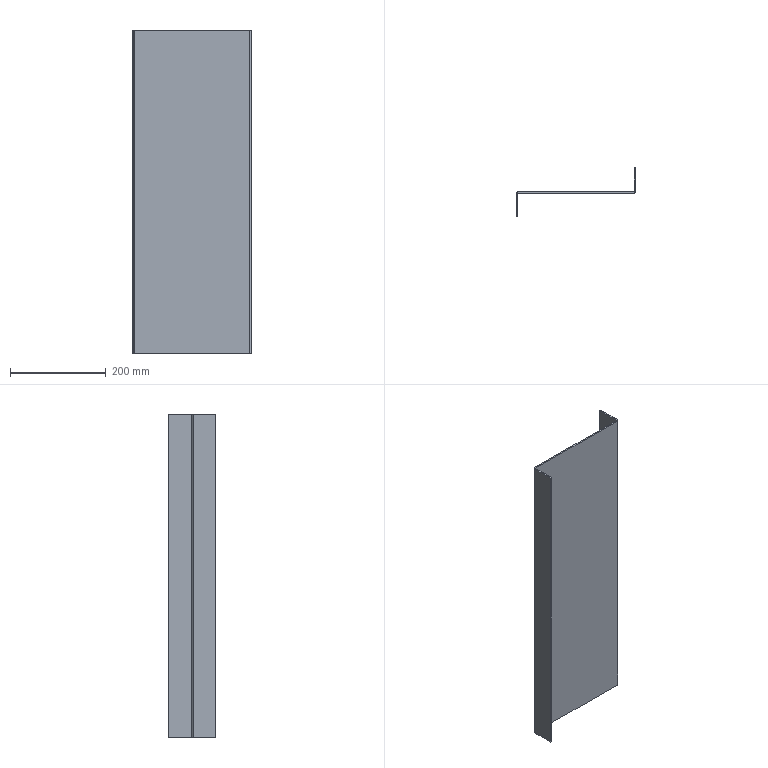Part | STEP file | 粉仓楼梯踏Plate 1 | 1 solid | 14 faces | box 248 x 100 x 674 mm | volume 693251 mm3 | plane 10 | cylinder 4 | commonest cylinder face diameters 2 x2 8 x2
STEP:
#1=CARTESIAN_POINT('',(0.,0.,0.));
#2=DIRECTION('',(0.,0.,1.));
#3=DIRECTION('',(1.,0.,0.));
#4=AXIS2_PLACEMENT_3D('',#1,#2,#3);
#5=CARTESIAN_POINT('',(3.,1.,-337.));
#6=VERTEX_POINT('',#5);
#7=CARTESIAN_POINT('',(3.,50.,-337.));
#8=VERTEX_POINT('',#7);
#9=CARTESIAN_POINT('',(3.,1.,-337.));
#10=DIRECTION('',(0.,1.,0.));
#11=VECTOR('',#10,1.);
#12=LINE('',#9,#11);
#13=CARTESIAN_POINT('',(3.,1.,337.));
#14=DIRECTION('',(-1.,0.,0.));
#15=DIRECTION('',(0.,0.,1.));
#16=AXIS2_PLACEMENT_3D('',#13,#14,#15);
#17=PLANE('',#16);
#18=CARTESIAN_POINT('',(-674.,0.));
#19=DIRECTION('',(0.,1.));
#20=VECTOR('',#19,1.);
#21=LINE('',#18,#20);
#22=(GEOMETRIC_REPRESENTATION_CONTEXT(2)PARAMETRIC_REPRESENTATION_CONTEXT()REPRESENTATION_CONTEXT('',''));
#23=DEFINITIONAL_REPRESENTATION('',(#21),#22);
#24=PCURVE('',#17,#23);
#25=CARTESIAN_POINT('',(-1.,1.,-337.));
#26=DIRECTION('',(0.,0.,1.));
#27=DIRECTION('',(1.,0.,0.));
#28=AXIS2_PLACEMENT_3D('',#25,#26,#27);
#29=PLANE('',#28);
#30=CARTESIAN_POINT('',(4.,0.));
#31=DIRECTION('',(0.,1.));
#32=VECTOR('',#31,1.);
#33=LINE('',#30,#32);
#34=(GEOMETRIC_REPRESENTATION_CONTEXT(2)PARAMETRIC_REPRESENTATION_CONTEXT()REPRESENTATION_CONTEXT('',''));
#35=DEFINITIONAL_REPRESENTATION('',(#33),#34);
#36=PCURVE('',#29,#35);
#37=SURFACE_CURVE('',#12,(#24,#36),.PCURVE_S1.);
#38=EDGE_CURVE('',#6,#8,#37,.T.);
#39=ORIENTED_EDGE('',*,*,#38,.T.);
#40=CARTESIAN_POINT('',(3.,50.,337.));
#41=VERTEX_POINT('',#40);
#42=CARTESIAN_POINT('',(3.,50.,337.));
#43=DIRECTION('',(0.,0.,-1.));
#44=VECTOR('',#43,1.);
#45=LINE('',#42,#44);
#46=CARTESIAN_POINT('',(0.,49.));
#47=DIRECTION('',(-1.,0.));
#48=VECTOR('',#47,1.);
#49=LINE('',#46,#48);
#50=(GEOMETRIC_REPRESENTATION_CONTEXT(2)PARAMETRIC_REPRESENTATION_CONTEXT()REPRESENTATION_CONTEXT('',''));
#51=DEFINITIONAL_REPRESENTATION('',(#49),#50);
#52=PCURVE('',#17,#51);
#53=CARTESIAN_POINT('',(0.,50.,337.));
#54=DIRECTION('',(0.,1.,0.));
#55=DIRECTION('',(0.,0.,1.));
#56=AXIS2_PLACEMENT_3D('',#53,#54,#55);
#57=PLANE('',#56);
#58=CARTESIAN_POINT('',(0.,3.));
#59=DIRECTION('',(-1.,0.));
#60=VECTOR('',#59,1.);
#61=LINE('',#58,#60);
#62=(GEOMETRIC_REPRESENTATION_CONTEXT(2)PARAMETRIC_REPRESENTATION_CONTEXT()REPRESENTATION_CONTEXT('',''));
#63=DEFINITIONAL_REPRESENTATION('',(#61),#62);
#64=PCURVE('',#57,#63);
#65=SURFACE_CURVE('',#45,(#52,#64),.PCURVE_S1.);
#66=EDGE_CURVE('',#41,#8,#65,.T.);
#67=ORIENTED_EDGE('',*,*,#66,.F.);
#68=CARTESIAN_POINT('',(3.,1.,337.));
#69=VERTEX_POINT('',#68);
#70=CARTESIAN_POINT('',(3.,1.,337.));
#71=DIRECTION('',(0.,1.,0.));
#72=VECTOR('',#71,1.);
#73=LINE('',#70,#72);
#74=CARTESIAN_POINT('',(0.,0.));
#75=DIRECTION('',(0.,1.));
#76=VECTOR('',#75,1.);
#77=LINE('',#74,#76);
#78=(GEOMETRIC_REPRESENTATION_CONTEXT(2)PARAMETRIC_REPRESENTATION_CONTEXT()REPRESENTATION_CONTEXT('',''));
#79=DEFINITIONAL_REPRESENTATION('',(#77),#78);
#80=PCURVE('',#17,#79);
#81=CARTESIAN_POINT('',(-1.,1.,337.));
#82=DIRECTION('',(0.,0.,1.));
#83=DIRECTION('',(1.,0.,0.));
#84=AXIS2_PLACEMENT_3D('',#81,#82,#83);
#85=PLANE('',#84);
#86=CARTESIAN_POINT('',(4.,0.));
#87=DIRECTION('',(0.,1.));
#88=VECTOR('',#87,1.);
#89=LINE('',#86,#88);
#90=(GEOMETRIC_REPRESENTATION_CONTEXT(2)PARAMETRIC_REPRESENTATION_CONTEXT()REPRESENTATION_CONTEXT('',''));
#91=DEFINITIONAL_REPRESENTATION('',(#89),#90);
#92=PCURVE('',#85,#91);
#93=SURFACE_CURVE('',#73,(#80,#92),.PCURVE_S1.);
#94=EDGE_CURVE('',#69,#41,#93,.T.);
#95=ORIENTED_EDGE('',*,*,#94,.F.);
#96=CARTESIAN_POINT('',(3.,1.,337.));
#97=DIRECTION('',(0.,0.,-1.));
#98=VECTOR('',#97,1.);
#99=LINE('',#96,#98);
#100=CARTESIAN_POINT('',(0.,0.));
#101=DIRECTION('',(-1.,0.));
#102=VECTOR('',#101,1.);
#103=LINE('',#100,#102);
#104=(GEOMETRIC_REPRESENTATION_CONTEXT(2)PARAMETRIC_REPRESENTATION_CONTEXT()REPRESENTATION_CONTEXT('',''));
#105=DEFINITIONAL_REPRESENTATION('',(#103),#104);
#106=PCURVE('',#17,#105);
#107=CARTESIAN_POINT('',(-1.,1.,337.));
#108=DIRECTION('',(0.,0.,-1.));
#109=DIRECTION('',(-1.,0.,0.));
#110=AXIS2_PLACEMENT_3D('',#107,#108,#109);
#111=CYLINDRICAL_SURFACE('',#110,4.);
#112=CARTESIAN_POINT('',(3.142,0.));
#113=DIRECTION('',(0.,1.));
#114=VECTOR('',#113,1.);
#115=LINE('',#112,#114);
#116=(GEOMETRIC_REPRESENTATION_CONTEXT(2)PARAMETRIC_REPRESENTATION_CONTEXT()REPRESENTATION_CONTEXT('',''));
#117=DEFINITIONAL_REPRESENTATION('',(#115),#116);
#118=PCURVE('',#111,#117);
#119=SURFACE_CURVE('',#99,(#106,#118),.PCURVE_S1.);
#120=EDGE_CURVE('',#69,#6,#119,.T.);
#121=ORIENTED_EDGE('',*,*,#120,.T.);
#122=EDGE_LOOP('',(#39,#67,#95,#121));
#123=FACE_BOUND('',#122,.T.);
#124=ADVANCED_FACE('',(#123),#17,.F.);
#125=CARTESIAN_POINT('',(0.,50.,-337.));
#126=VERTEX_POINT('',#125);
#127=CARTESIAN_POINT('',(0.,50.,-337.));
#128=DIRECTION('',(1.,0.,0.));
#129=VECTOR('',#128,1.);
#130=LINE('',#127,#129);
#131=CARTESIAN_POINT('',(-674.,0.));
#132=DIRECTION('',(0.,1.));
#133=VECTOR('',#132,1.);
#134=LINE('',#131,#133);
#135=(GEOMETRIC_REPRESENTATION_CONTEXT(2)PARAMETRIC_REPRESENTATION_CONTEXT()REPRESENTATION_CONTEXT('',''));
#136=DEFINITIONAL_REPRESENTATION('',(#134),#135);
#137=PCURVE('',#57,#136);
#138=CARTESIAN_POINT('',(1.,49.));
#139=DIRECTION('',(1.,0.));
#140=VECTOR('',#139,1.);
#141=LINE('',#138,#140);
#142=(GEOMETRIC_REPRESENTATION_CONTEXT(2)PARAMETRIC_REPRESENTATION_CONTEXT()REPRESENTATION_CONTEXT('',''));
#143=DEFINITIONAL_REPRESENTATION('',(#141),#142);
#144=PCURVE('',#29,#143);
#145=SURFACE_CURVE('',#130,(#137,#144),.PCURVE_S1.);
#146=EDGE_CURVE('',#126,#8,#145,.T.);
#147=ORIENTED_EDGE('',*,*,#146,.F.);
#148=CARTESIAN_POINT('',(0.,50.,337.));
#149=VERTEX_POINT('',#148);
#150=CARTESIAN_POINT('',(0.,50.,337.));
#151=DIRECTION('',(0.,0.,-1.));
#152=VECTOR('',#151,1.);
#153=LINE('',#150,#152);
#154=CARTESIAN_POINT('',(0.,0.));
#155=DIRECTION('',(-1.,0.));
#156=VECTOR('',#155,1.);
#157=LINE('',#154,#156);
#158=(GEOMETRIC_REPRESENTATION_CONTEXT(2)PARAMETRIC_REPRESENTATION_CONTEXT()REPRESENTATION_CONTEXT('',''));
#159=DEFINITIONAL_REPRESENTATION('',(#157),#158);
#160=PCURVE('',#57,#159);
#161=CARTESIAN_POINT('',(0.,1.,337.));
#162=DIRECTION('',(-1.,0.,0.));
#163=DIRECTION('',(0.,0.,1.));
#164=AXIS2_PLACEMENT_3D('',#161,#162,#163);
#165=PLANE('',#164);
#166=CARTESIAN_POINT('',(0.,49.));
#167=DIRECTION('',(-1.,0.));
#168=VECTOR('',#167,1.);
#169=LINE('',#166,#168);
#170=(GEOMETRIC_REPRESENTATION_CONTEXT(2)PARAMETRIC_REPRESENTATION_CONTEXT()REPRESENTATION_CONTEXT('',''));
#171=DEFINITIONAL_REPRESENTATION('',(#169),#170);
#172=PCURVE('',#165,#171);
#173=SURFACE_CURVE('',#153,(#160,#172),.PCURVE_S1.);
#174=EDGE_CURVE('',#149,#126,#173,.T.);
#175=ORIENTED_EDGE('',*,*,#174,.F.);
#176=CARTESIAN_POINT('',(0.,50.,337.));
#177=DIRECTION('',(1.,0.,0.));
#178=VECTOR('',#177,1.);
#179=LINE('',#176,#178);
#180=CARTESIAN_POINT('',(0.,0.));
#181=DIRECTION('',(0.,1.));
#182=VECTOR('',#181,1.);
#183=LINE('',#180,#182);
#184=(GEOMETRIC_REPRESENTATION_CONTEXT(2)PARAMETRIC_REPRESENTATION_CONTEXT()REPRESENTATION_CONTEXT('',''));
#185=DEFINITIONAL_REPRESENTATION('',(#183),#184);
#186=PCURVE('',#57,#185);
#187=CARTESIAN_POINT('',(1.,49.));
#188=DIRECTION('',(1.,0.));
#189=VECTOR('',#188,1.);
#190=LINE('',#187,#189);
#191=(GEOMETRIC_REPRESENTATION_CONTEXT(2)PARAMETRIC_REPRESENTATION_CONTEXT()REPRESENTATION_CONTEXT('',''));
#192=DEFINITIONAL_REPRESENTATION('',(#190),#191);
#193=PCURVE('',#85,#192);
#194=SURFACE_CURVE('',#179,(#186,#193),.PCURVE_S1.);
#195=EDGE_CURVE('',#149,#41,#194,.T.);
#196=ORIENTED_EDGE('',*,*,#195,.T.);
#197=ORIENTED_EDGE('',*,*,#66,.T.);
#198=EDGE_LOOP('',(#147,#175,#196,#197));
#199=FACE_BOUND('',#198,.T.);
#200=ADVANCED_FACE('',(#199),#57,.T.);
#201=CARTESIAN_POINT('',(0.,1.,-337.));
#202=VERTEX_POINT('',#201);
#203=CARTESIAN_POINT('',(0.,1.,-337.));
#204=DIRECTION('',(0.,1.,0.));
#205=VECTOR('',#204,1.);
#206=LINE('',#203,#205);
#207=CARTESIAN_POINT('',(-674.,0.));
#208=DIRECTION('',(0.,1.));
#209=VECTOR('',#208,1.);
#210=LINE('',#207,#209);
#211=(GEOMETRIC_REPRESENTATION_CONTEXT(2)PARAMETRIC_REPRESENTATION_CONTEXT()REPRESENTATION_CONTEXT('',''));
#212=DEFINITIONAL_REPRESENTATION('',(#210),#211);
#213=PCURVE('',#165,#212);
#214=CARTESIAN_POINT('',(1.,0.));
#215=DIRECTION('',(0.,1.));
#216=VECTOR('',#215,1.);
#217=LINE('',#214,#216);
#218=(GEOMETRIC_REPRESENTATION_CONTEXT(2)PARAMETRIC_REPRESENTATION_CONTEXT()REPRESENTATION_CONTEXT('',''));
#219=DEFINITIONAL_REPRESENTATION('',(#217),#218);
#220=PCURVE('',#29,#219);
#221=SURFACE_CURVE('',#206,(#213,#220),.PCURVE_S1.);
#222=EDGE_CURVE('',#202,#126,#221,.T.);
#223=ORIENTED_EDGE('',*,*,#222,.F.);
#224=CARTESIAN_POINT('',(0.,1.,337.));
#225=VERTEX_POINT('',#224);
#226=CARTESIAN_POINT('',(0.,1.,337.));
#227=DIRECTION('',(0.,0.,-1.));
#228=VECTOR('',#227,1.);
#229=LINE('',#226,#228);
#230=CARTESIAN_POINT('',(0.,0.));
#231=DIRECTION('',(-1.,0.));
#232=VECTOR('',#231,1.);
#233=LINE('',#230,#232);
#234=(GEOMETRIC_REPRESENTATION_CONTEXT(2)PARAMETRIC_REPRESENTATION_CONTEXT()REPRESENTATION_CONTEXT('',''));
#235=DEFINITIONAL_REPRESENTATION('',(#233),#234);
#236=PCURVE('',#165,#235);
#237=CARTESIAN_POINT('',(-1.,1.,337.));
#238=DIRECTION('',(0.,0.,-1.));
#239=DIRECTION('',(-1.,0.,0.));
#240=AXIS2_PLACEMENT_3D('',#237,#238,#239);
#241=CYLINDRICAL_SURFACE('',#240,1.);
#242=CARTESIAN_POINT('',(3.142,0.));
#243=DIRECTION('',(0.,1.));
#244=VECTOR('',#243,1.);
#245=LINE('',#242,#244);
#246=(GEOMETRIC_REPRESENTATION_CONTEXT(2)PARAMETRIC_REPRESENTATION_CONTEXT()REPRESENTATION_CONTEXT('',''));
#247=DEFINITIONAL_REPRESENTATION('',(#245),#246);
#248=PCURVE('',#241,#247);
#249=SURFACE_CURVE('',#229,(#236,#248),.PCURVE_S1.);
#250=EDGE_CURVE('',#225,#202,#249,.T.);
#251=ORIENTED_EDGE('',*,*,#250,.F.);
#252=CARTESIAN_POINT('',(0.,1.,337.));
#253=DIRECTION('',(0.,1.,0.));
#254=VECTOR('',#253,1.);
#255=LINE('',#252,#254);
#256=CARTESIAN_POINT('',(0.,0.));
#257=DIRECTION('',(0.,1.));
#258=VECTOR('',#257,1.);
#259=LINE('',#256,#258);
#260=(GEOMETRIC_REPRESENTATION_CONTEXT(2)PARAMETRIC_REPRESENTATION_CONTEXT()REPRESENTATION_CONTEXT('',''));
#261=DEFINITIONAL_REPRESENTATION('',(#259),#260);
#262=PCURVE('',#165,#261);
#263=CARTESIAN_POINT('',(1.,0.));
#264=DIRECTION('',(0.,1.));
#265=VECTOR('',#264,1.);
#266=LINE('',#263,#265);
#267=(GEOMETRIC_REPRESENTATION_CONTEXT(2)PARAMETRIC_REPRESENTATION_CONTEXT()REPRESENTATION_CONTEXT('',''));
#268=DEFINITIONAL_REPRESENTATION('',(#266),#267);
#269=PCURVE('',#85,#268);
#270=SURFACE_CURVE('',#255,(#262,#269),.PCURVE_S1.);
#271=EDGE_CURVE('',#225,#149,#270,.T.);
#272=ORIENTED_EDGE('',*,*,#271,.T.);
#273=ORIENTED_EDGE('',*,*,#174,.T.);
#274=EDGE_LOOP('',(#223,#251,#272,#273));
#275=FACE_BOUND('',#274,.T.);
#276=ADVANCED_FACE('',(#275),#165,.T.);
#277=ORIENTED_EDGE('',*,*,#250,.F.);
#278=CARTESIAN_POINT('',(-1.,0.,337.));
#279=VERTEX_POINT('',#278);
#280=CARTESIAN_POINT('',(-1.,1.,337.));
#281=DIRECTION('',(0.,0.,1.));
#282=DIRECTION('',(1.,0.,0.));
#283=AXIS2_PLACEMENT_3D('',#280,#281,#282);
#284=CIRCLE('',#283,1.);
#285=CARTESIAN_POINT('',(9.425,0.));
#286=DIRECTION('',(-1.,0.));
#287=VECTOR('',#286,1.);
#288=LINE('',#285,#287);
#289=(GEOMETRIC_REPRESENTATION_CONTEXT(2)PARAMETRIC_REPRESENTATION_CONTEXT()REPRESENTATION_CONTEXT('',''));
#290=DEFINITIONAL_REPRESENTATION('',(#288),#289);
#291=PCURVE('',#241,#290);
#292=CARTESIAN_POINT('',(0.,0.));
#293=DIRECTION('',(1.,0.));
#294=AXIS2_PLACEMENT_2D('',#292,#293);
#295=CIRCLE('',#294,1.);
#296=(GEOMETRIC_REPRESENTATION_CONTEXT(2)PARAMETRIC_REPRESENTATION_CONTEXT()REPRESENTATION_CONTEXT('',''));
#297=DEFINITIONAL_REPRESENTATION('',(#295),#296);
#298=PCURVE('',#85,#297);
#299=SURFACE_CURVE('',#284,(#291,#298),.PCURVE_S1.);
#300=EDGE_CURVE('',#279,#225,#299,.T.);
#301=ORIENTED_EDGE('',*,*,#300,.F.);
#302=CARTESIAN_POINT('',(-1.,0.,-337.));
#303=VERTEX_POINT('',#302);
#304=CARTESIAN_POINT('',(-1.,0.,337.));
#305=DIRECTION('',(0.,0.,-1.));
#306=VECTOR('',#305,1.);
#307=LINE('',#304,#306);
#308=CARTESIAN_POINT('',(4.712,0.));
#309=DIRECTION('',(0.,1.));
#310=VECTOR('',#309,1.);
#311=LINE('',#308,#310);
#312=(GEOMETRIC_REPRESENTATION_CONTEXT(2)PARAMETRIC_REPRESENTATION_CONTEXT()REPRESENTATION_CONTEXT('',''));
#313=DEFINITIONAL_REPRESENTATION('',(#311),#312);
#314=PCURVE('',#241,#313);
#315=CARTESIAN_POINT('',(-241.,0.,337.));
#316=DIRECTION('',(0.,1.,0.));
#317=DIRECTION('',(0.,0.,1.));
#318=AXIS2_PLACEMENT_3D('',#315,#316,#317);
#319=PLANE('',#318);
#320=CARTESIAN_POINT('',(0.,240.));
#321=DIRECTION('',(-1.,0.));
#322=VECTOR('',#321,1.);
#323=LINE('',#320,#322);
#324=(GEOMETRIC_REPRESENTATION_CONTEXT(2)PARAMETRIC_REPRESENTATION_CONTEXT()REPRESENTATION_CONTEXT('',''));
#325=DEFINITIONAL_REPRESENTATION('',(#323),#324);
#326=PCURVE('',#319,#325);
#327=SURFACE_CURVE('',#307,(#314,#326),.PCURVE_S1.);
#328=EDGE_CURVE('',#279,#303,#327,.T.);
#329=ORIENTED_EDGE('',*,*,#328,.T.);
#330=CARTESIAN_POINT('',(-1.,1.,-337.));
#331=DIRECTION('',(0.,0.,1.));
#332=DIRECTION('',(1.,0.,0.));
#333=AXIS2_PLACEMENT_3D('',#330,#331,#332);
#334=CIRCLE('',#333,1.);
#335=CARTESIAN_POINT('',(9.425,674.));
#336=DIRECTION('',(-1.,0.));
#337=VECTOR('',#336,1.);
#338=LINE('',#335,#337);
#339=(GEOMETRIC_REPRESENTATION_CONTEXT(2)PARAMETRIC_REPRESENTATION_CONTEXT()REPRESENTATION_CONTEXT('',''));
#340=DEFINITIONAL_REPRESENTATION('',(#338),#339);
#341=PCURVE('',#241,#340);
#342=CARTESIAN_POINT('',(0.,0.));
#343=DIRECTION('',(1.,0.));
#344=AXIS2_PLACEMENT_2D('',#342,#343);
#345=CIRCLE('',#344,1.);
#346=(GEOMETRIC_REPRESENTATION_CONTEXT(2)PARAMETRIC_REPRESENTATION_CONTEXT()REPRESENTATION_CONTEXT('',''));
#347=DEFINITIONAL_REPRESENTATION('',(#345),#346);
#348=PCURVE('',#29,#347);
#349=SURFACE_CURVE('',#334,(#341,#348),.PCURVE_S1.);
#350=EDGE_CURVE('',#303,#202,#349,.T.);
#351=ORIENTED_EDGE('',*,*,#350,.T.);
#352=EDGE_LOOP('',(#277,#301,#329,#351));
#353=FACE_BOUND('',#352,.F.);
#354=ADVANCED_FACE('',(#353),#241,.F.);
#355=CARTESIAN_POINT('',(-241.,0.,-337.));
#356=VERTEX_POINT('',#355);
#357=CARTESIAN_POINT('',(-241.,0.,-337.));
#358=DIRECTION('',(1.,0.,0.));
#359=VECTOR('',#358,1.);
#360=LINE('',#357,#359);
#361=CARTESIAN_POINT('',(-674.,0.));
#362=DIRECTION('',(0.,1.));
#363=VECTOR('',#362,1.);
#364=LINE('',#361,#363);
#365=(GEOMETRIC_REPRESENTATION_CONTEXT(2)PARAMETRIC_REPRESENTATION_CONTEXT()REPRESENTATION_CONTEXT('',''));
#366=DEFINITIONAL_REPRESENTATION('',(#364),#365);
#367=PCURVE('',#319,#366);
#368=CARTESIAN_POINT('',(-240.,-1.));
#369=DIRECTION('',(1.,0.));
#370=VECTOR('',#369,1.);
#371=LINE('',#368,#370);
#372=(GEOMETRIC_REPRESENTATION_CONTEXT(2)PARAMETRIC_REPRESENTATION_CONTEXT()REPRESENTATION_CONTEXT('',''));
#373=DEFINITIONAL_REPRESENTATION('',(#371),#372);
#374=PCURVE('',#29,#373);
#375=SURFACE_CURVE('',#360,(#367,#374),.PCURVE_S1.);
#376=EDGE_CURVE('',#356,#303,#375,.T.);
#377=ORIENTED_EDGE('',*,*,#376,.F.);
#378=CARTESIAN_POINT('',(-241.,0.,337.));
#379=VERTEX_POINT('',#378);
#380=CARTESIAN_POINT('',(-241.,0.,337.));
#381=DIRECTION('',(0.,0.,-1.));
#382=VECTOR('',#381,1.);
#383=LINE('',#380,#382);
#384=CARTESIAN_POINT('',(0.,0.));
#385=DIRECTION('',(-1.,0.));
#386=VECTOR('',#385,1.);
#387=LINE('',#384,#386);
#388=(GEOMETRIC_REPRESENTATION_CONTEXT(2)PARAMETRIC_REPRESENTATION_CONTEXT()REPRESENTATION_CONTEXT('',''));
#389=DEFINITIONAL_REPRESENTATION('',(#387),#388);
#390=PCURVE('',#319,#389);
#391=CARTESIAN_POINT('',(-241.,-4.,337.));
#392=DIRECTION('',(0.,0.,-1.));
#393=DIRECTION('',(-1.,0.,0.));
#394=AXIS2_PLACEMENT_3D('',#391,#392,#393);
#395=CYLINDRICAL_SURFACE('',#394,4.);
#396=CARTESIAN_POINT('',(1.571,0.));
#397=DIRECTION('',(0.,1.));
#398=VECTOR('',#397,1.);
#399=LINE('',#396,#398);
#400=(GEOMETRIC_REPRESENTATION_CONTEXT(2)PARAMETRIC_REPRESENTATION_CONTEXT()REPRESENTATION_CONTEXT('',''));
#401=DEFINITIONAL_REPRESENTATION('',(#399),#400);
#402=PCURVE('',#395,#401);
#403=SURFACE_CURVE('',#383,(#390,#402),.PCURVE_S1.);
#404=EDGE_CURVE('',#379,#356,#403,.T.);
#405=ORIENTED_EDGE('',*,*,#404,.F.);
#406=CARTESIAN_POINT('',(-241.,0.,337.));
#407=DIRECTION('',(1.,0.,0.));
#408=VECTOR('',#407,1.);
#409=LINE('',#406,#408);
#410=CARTESIAN_POINT('',(0.,0.));
#411=DIRECTION('',(0.,1.));
#412=VECTOR('',#411,1.);
#413=LINE('',#410,#412);
#414=(GEOMETRIC_REPRESENTATION_CONTEXT(2)PARAMETRIC_REPRESENTATION_CONTEXT()REPRESENTATION_CONTEXT('',''));
#415=DEFINITIONAL_REPRESENTATION('',(#413),#414);
#416=PCURVE('',#319,#415);
#417=CARTESIAN_POINT('',(-240.,-1.));
#418=DIRECTION('',(1.,0.));
#419=VECTOR('',#418,1.);
#420=LINE('',#417,#419);
#421=(GEOMETRIC_REPRESENTATION_CONTEXT(2)PARAMETRIC_REPRESENTATION_CONTEXT()REPRESENTATION_CONTEXT('',''));
#422=DEFINITIONAL_REPRESENTATION('',(#420),#421);
#423=PCURVE('',#85,#422);
#424=SURFACE_CURVE('',#409,(#416,#423),.PCURVE_S1.);
#425=EDGE_CURVE('',#379,#279,#424,.T.);
#426=ORIENTED_EDGE('',*,*,#425,.T.);
#427=ORIENTED_EDGE('',*,*,#328,.T.);
#428=EDGE_LOOP('',(#377,#405,#426,#427));
#429=FACE_BOUND('',#428,.T.);
#430=ADVANCED_FACE('',(#429),#319,.T.);
#431=CARTESIAN_POINT('',(-245.,-4.,-337.));
#432=VERTEX_POINT('',#431);
#433=CARTESIAN_POINT('',(-241.,-4.,-337.));
#434=DIRECTION('',(0.,0.,-1.));
#435=DIRECTION('',(1.,0.,0.));
#436=AXIS2_PLACEMENT_3D('',#433,#434,#435);
#437=CIRCLE('',#436,4.);
#438=CARTESIAN_POINT('',(-3.142,674.));
#439=DIRECTION('',(1.,0.));
#440=VECTOR('',#439,1.);
#441=LINE('',#438,#440);
#442=(GEOMETRIC_REPRESENTATION_CONTEXT(2)PARAMETRIC_REPRESENTATION_CONTEXT()REPRESENTATION_CONTEXT('',''));
#443=DEFINITIONAL_REPRESENTATION('',(#441),#442);
#444=PCURVE('',#395,#443);
#445=CARTESIAN_POINT('',(-236.,-5.));
#446=CARTESIAN_POINT('',(-236.,-11.928));
#447=CARTESIAN_POINT('',(-242.,-8.464));
#448=CARTESIAN_POINT('',(-248.,-5.));
#449=CARTESIAN_POINT('',(-242.,-1.536));
#450=CARTESIAN_POINT('',(-236.,1.928));
#451=CARTESIAN_POINT('',(-236.,-5.));
#452=(BOUNDED_CURVE()B_SPLINE_CURVE(2,(#445,#446,#447,#448,#449,#450,#451),.UNSPECIFIED.,.T.,.F.)B_SPLINE_CURVE_WITH_KNOTS((1,2,2,2,2,1),(-2.094,0.,2.094,4.189,6.283,8.378),.UNSPECIFIED.)CURVE()GEOMETRIC_REPRESENTATION_ITEM()RATIONAL_B_SPLINE_CURVE((1.,0.5,1.,0.5,1.,0.5,1.))REPRESENTATION_ITEM(''));
#453=(GEOMETRIC_REPRESENTATION_CONTEXT(2)PARAMETRIC_REPRESENTATION_CONTEXT()REPRESENTATION_CONTEXT('',''));
#454=DEFINITIONAL_REPRESENTATION('',(#452),#453);
#455=PCURVE('',#29,#454);
#456=SURFACE_CURVE('',#437,(#444,#455),.PCURVE_S1.);
#457=EDGE_CURVE('',#432,#356,#456,.T.);
#458=ORIENTED_EDGE('',*,*,#457,.F.);
#459=CARTESIAN_POINT('',(-245.,-4.,337.));
#460=VERTEX_POINT('',#459);
#461=CARTESIAN_POINT('',(-245.,-4.,337.));
#462=DIRECTION('',(0.,0.,-1.));
#463=VECTOR('',#462,1.);
#464=LINE('',#461,#463);
#465=CARTESIAN_POINT('',(0.,0.));
#466=DIRECTION('',(0.,1.));
#467=VECTOR('',#466,1.);
#468=LINE('',#465,#467);
#469=(GEOMETRIC_REPRESENTATION_CONTEXT(2)PARAMETRIC_REPRESENTATION_CONTEXT()REPRESENTATION_CONTEXT('',''));
#470=DEFINITIONAL_REPRESENTATION('',(#468),#469);
#471=PCURVE('',#395,#470);
#472=CARTESIAN_POINT('',(-245.,-4.,337.));
#473=DIRECTION('',(-1.,0.,0.));
#474=DIRECTION('',(0.,0.,1.));
#475=AXIS2_PLACEMENT_3D('',#472,#473,#474);
#476=PLANE('',#475);
#477=CARTESIAN_POINT('',(0.,0.));
#478=DIRECTION('',(-1.,0.));
#479=VECTOR('',#478,1.);
#480=LINE('',#477,#479);
#481=(GEOMETRIC_REPRESENTATION_CONTEXT(2)PARAMETRIC_REPRESENTATION_CONTEXT()REPRESENTATION_CONTEXT('',''));
#482=DEFINITIONAL_REPRESENTATION('',(#480),#481);
#483=PCURVE('',#476,#482);
#484=SURFACE_CURVE('',#464,(#471,#483),.PCURVE_S1.);
#485=EDGE_CURVE('',#460,#432,#484,.T.);
#486=ORIENTED_EDGE('',*,*,#485,.F.);
#487=CARTESIAN_POINT('',(-241.,-4.,337.));
#488=DIRECTION('',(0.,0.,-1.));
#489=DIRECTION('',(1.,0.,0.));
#490=AXIS2_PLACEMENT_3D('',#487,#488,#489);
#491=CIRCLE('',#490,4.);
#492=CARTESIAN_POINT('',(-3.142,0.));
#493=DIRECTION('',(1.,0.));
#494=VECTOR('',#493,1.);
#495=LINE('',#492,#494);
#496=(GEOMETRIC_REPRESENTATION_CONTEXT(2)PARAMETRIC_REPRESENTATION_CONTEXT()REPRESENTATION_CONTEXT('',''));
#497=DEFINITIONAL_REPRESENTATION('',(#495),#496);
#498=PCURVE('',#395,#497);
#499=CARTESIAN_POINT('',(-236.,-5.));
#500=CARTESIAN_POINT('',(-236.,-11.928));
#501=CARTESIAN_POINT('',(-242.,-8.464));
#502=CARTESIAN_POINT('',(-248.,-5.));
#503=CARTESIAN_POINT('',(-242.,-1.536));
#504=CARTESIAN_POINT('',(-236.,1.928));
#505=CARTESIAN_POINT('',(-236.,-5.));
#506=(BOUNDED_CURVE()B_SPLINE_CURVE(2,(#499,#500,#501,#502,#503,#504,#505),.UNSPECIFIED.,.T.,.F.)B_SPLINE_CURVE_WITH_KNOTS((1,2,2,2,2,1),(-2.094,0.,2.094,4.189,6.283,8.378),.UNSPECIFIED.)CURVE()GEOMETRIC_REPRESENTATION_ITEM()RATIONAL_B_SPLINE_CURVE((1.,0.5,1.,0.5,1.,0.5,1.))REPRESENTATION_ITEM(''));
#507=(GEOMETRIC_REPRESENTATION_CONTEXT(2)PARAMETRIC_REPRESENTATION_CONTEXT()REPRESENTATION_CONTEXT('',''));
#508=DEFINITIONAL_REPRESENTATION('',(#506),#507);
#509=PCURVE('',#85,#508);
#510=SURFACE_CURVE('',#491,(#498,#509),.PCURVE_S1.);
#511=EDGE_CURVE('',#460,#379,#510,.T.);
#512=ORIENTED_EDGE('',*,*,#511,.T.);
#513=ORIENTED_EDGE('',*,*,#404,.T.);
#514=EDGE_LOOP('',(#458,#486,#512,#513));
#515=FACE_BOUND('',#514,.T.);
#516=ADVANCED_FACE('',(#515),#395,.T.);
#517=CARTESIAN_POINT('',(-245.,-50.,-337.));
#518=VERTEX_POINT('',#517);
#519=CARTESIAN_POINT('',(-245.,-4.,-337.));
#520=DIRECTION('',(0.,1.,0.));
#521=VECTOR('',#520,1.);
#522=LINE('',#519,#521);
#523=CARTESIAN_POINT('',(-674.,0.));
#524=DIRECTION('',(0.,1.));
#525=VECTOR('',#524,1.);
#526=LINE('',#523,#525);
#527=(GEOMETRIC_REPRESENTATION_CONTEXT(2)PARAMETRIC_REPRESENTATION_CONTEXT()REPRESENTATION_CONTEXT('',''));
#528=DEFINITIONAL_REPRESENTATION('',(#526),#527);
#529=PCURVE('',#476,#528);
#530=CARTESIAN_POINT('',(-244.,-5.));
#531=DIRECTION('',(0.,1.));
#532=VECTOR('',#531,1.);
#533=LINE('',#530,#532);
#534=(GEOMETRIC_REPRESENTATION_CONTEXT(2)PARAMETRIC_REPRESENTATION_CONTEXT()REPRESENTATION_CONTEXT('',''));
#535=DEFINITIONAL_REPRESENTATION('',(#533),#534);
#536=PCURVE('',#29,#535);
#537=SURFACE_CURVE('',#522,(#529,#536),.PCURVE_S1.);
#538=EDGE_CURVE('',#518,#432,#537,.T.);
#539=ORIENTED_EDGE('',*,*,#538,.F.);
#540=CARTESIAN_POINT('',(-245.,-50.,337.));
#541=VERTEX_POINT('',#540);
#542=CARTESIAN_POINT('',(-245.,-50.,337.));
#543=DIRECTION('',(0.,0.,-1.));
#544=VECTOR('',#543,1.);
#545=LINE('',#542,#544);
#546=CARTESIAN_POINT('',(0.,-46.));
#547=DIRECTION('',(-1.,0.));
#548=VECTOR('',#547,1.);
#549=LINE('',#546,#548);
#550=(GEOMETRIC_REPRESENTATION_CONTEXT(2)PARAMETRIC_REPRESENTATION_CONTEXT()REPRESENTATION_CONTEXT('',''));
#551=DEFINITIONAL_REPRESENTATION('',(#549),#550);
#552=PCURVE('',#476,#551);
#553=CARTESIAN_POINT('',(-242.,-50.,337.));
#554=DIRECTION('',(0.,-1.,0.));
#555=DIRECTION('',(0.,0.,-1.));
#556=AXIS2_PLACEMENT_3D('',#553,#554,#555);
#557=PLANE('',#556);
#558=CARTESIAN_POINT('',(0.,-3.));
#559=DIRECTION('',(1.,0.));
#560=VECTOR('',#559,1.);
#561=LINE('',#558,#560);
#562=(GEOMETRIC_REPRESENTATION_CONTEXT(2)PARAMETRIC_REPRESENTATION_CONTEXT()REPRESENTATION_CONTEXT('',''));
#563=DEFINITIONAL_REPRESENTATION('',(#561),#562);
#564=PCURVE('',#557,#563);
#565=SURFACE_CURVE('',#545,(#552,#564),.PCURVE_S1.);
#566=EDGE_CURVE('',#541,#518,#565,.T.);
#567=ORIENTED_EDGE('',*,*,#566,.F.);
#568=CARTESIAN_POINT('',(-245.,-4.,337.));
#569=DIRECTION('',(0.,1.,0.));
#570=VECTOR('',#569,1.);
#571=LINE('',#568,#570);
#572=CARTESIAN_POINT('',(0.,0.));
#573=DIRECTION('',(0.,1.));
#574=VECTOR('',#573,1.);
#575=LINE('',#572,#574);
#576=(GEOMETRIC_REPRESENTATION_CONTEXT(2)PARAMETRIC_REPRESENTATION_CONTEXT()REPRESENTATION_CONTEXT('',''));
#577=DEFINITIONAL_REPRESENTATION('',(#575),#576);
#578=PCURVE('',#476,#577);
#579=CARTESIAN_POINT('',(-244.,-5.));
#580=DIRECTION('',(0.,1.));
#581=VECTOR('',#580,1.);
#582=LINE('',#579,#581);
#583=(GEOMETRIC_REPRESENTATION_CONTEXT(2)PARAMETRIC_REPRESENTATION_CONTEXT()REPRESENTATION_CONTEXT('',''));
#584=DEFINITIONAL_REPRESENTATION('',(#582),#583);
#585=PCURVE('',#85,#584);
#586=SURFACE_CURVE('',#571,(#578,#585),.PCURVE_S1.);
#587=EDGE_CURVE('',#541,#460,#586,.T.);
#588=ORIENTED_EDGE('',*,*,#587,.T.);
#589=ORIENTED_EDGE('',*,*,#485,.T.);
#590=EDGE_LOOP('',(#539,#567,#588,#589));
#591=FACE_BOUND('',#590,.T.);
#592=ADVANCED_FACE('',(#591),#476,.T.);
#593=CARTESIAN_POINT('',(-242.,-50.,-337.));
#594=VERTEX_POINT('',#593);
#595=CARTESIAN_POINT('',(-242.,-50.,-337.));
#596=DIRECTION('',(-1.,0.,0.));
#597=VECTOR('',#596,1.);
#598=LINE('',#595,#597);
#599=CARTESIAN_POINT('',(674.,0.));
#600=DIRECTION('',(0.,-1.));
#601=VECTOR('',#600,1.);
#602=LINE('',#599,#601);
#603=(GEOMETRIC_REPRESENTATION_CONTEXT(2)PARAMETRIC_REPRESENTATION_CONTEXT()REPRESENTATION_CONTEXT('',''));
#604=DEFINITIONAL_REPRESENTATION('',(#602),#603);
#605=PCURVE('',#557,#604);
#606=CARTESIAN_POINT('',(-241.,-51.));
#607=DIRECTION('',(-1.,0.));
#608=VECTOR('',#607,1.);
#609=LINE('',#606,#608);
#610=(GEOMETRIC_REPRESENTATION_CONTEXT(2)PARAMETRIC_REPRESENTATION_CONTEXT()REPRESENTATION_CONTEXT('',''));
#611=DEFINITIONAL_REPRESENTATION('',(#609),#610);
#612=PCURVE('',#29,#611);
#613=SURFACE_CURVE('',#598,(#605,#612),.PCURVE_S1.);
#614=EDGE_CURVE('',#594,#518,#613,.T.);
#615=ORIENTED_EDGE('',*,*,#614,.F.);
#616=CARTESIAN_POINT('',(-242.,-50.,337.));
#617=VERTEX_POINT('',#616);
#618=CARTESIAN_POINT('',(-242.,-50.,337.));
#619=DIRECTION('',(0.,0.,-1.));
#620=VECTOR('',#619,1.);
#621=LINE('',#618,#620);
#622=CARTESIAN_POINT('',(0.,0.));
#623=DIRECTION('',(1.,0.));
#624=VECTOR('',#623,1.);
#625=LINE('',#622,#624);
#626=(GEOMETRIC_REPRESENTATION_CONTEXT(2)PARAMETRIC_REPRESENTATION_CONTEXT()REPRESENTATION_CONTEXT('',''));
#627=DEFINITIONAL_REPRESENTATION('',(#625),#626);
#628=PCURVE('',#557,#627);
#629=CARTESIAN_POINT('',(-242.,-4.,337.));
#630=DIRECTION('',(-1.,0.,0.));
#631=DIRECTION('',(0.,0.,1.));
#632=AXIS2_PLACEMENT_3D('',#629,#630,#631);
#633=PLANE('',#632);
#634=CARTESIAN_POINT('',(0.,-46.));
#635=DIRECTION('',(-1.,0.));
#636=VECTOR('',#635,1.);
#637=LINE('',#634,#636);
#638=(GEOMETRIC_REPRESENTATION_CONTEXT(2)PARAMETRIC_REPRESENTATION_CONTEXT()REPRESENTATION_CONTEXT('',''));
#639=DEFINITIONAL_REPRESENTATION('',(#637),#638);
#640=PCURVE('',#633,#639);
#641=SURFACE_CURVE('',#621,(#628,#640),.PCURVE_S1.);
#642=EDGE_CURVE('',#617,#594,#641,.T.);
#643=ORIENTED_EDGE('',*,*,#642,.F.);
#644=CARTESIAN_POINT('',(-242.,-50.,337.));
#645=DIRECTION('',(-1.,0.,0.));
#646=VECTOR('',#645,1.);
#647=LINE('',#644,#646);
#648=CARTESIAN_POINT('',(0.,0.));
#649=DIRECTION('',(0.,-1.));
#650=VECTOR('',#649,1.);
#651=LINE('',#648,#650);
#652=(GEOMETRIC_REPRESENTATION_CONTEXT(2)PARAMETRIC_REPRESENTATION_CONTEXT()REPRESENTATION_CONTEXT('',''));
#653=DEFINITIONAL_REPRESENTATION('',(#651),#652);
#654=PCURVE('',#557,#653);
#655=CARTESIAN_POINT('',(-241.,-51.));
#656=DIRECTION('',(-1.,0.));
#657=VECTOR('',#656,1.);
#658=LINE('',#655,#657);
#659=(GEOMETRIC_REPRESENTATION_CONTEXT(2)PARAMETRIC_REPRESENTATION_CONTEXT()REPRESENTATION_CONTEXT('',''));
#660=DEFINITIONAL_REPRESENTATION('',(#658),#659);
#661=PCURVE('',#85,#660);
#662=SURFACE_CURVE('',#647,(#654,#661),.PCURVE_S1.);
#663=EDGE_CURVE('',#617,#541,#662,.T.);
#664=ORIENTED_EDGE('',*,*,#663,.T.);
#665=ORIENTED_EDGE('',*,*,#566,.T.);
#666=EDGE_LOOP('',(#615,#643,#664,#665));
#667=FACE_BOUND('',#666,.T.);
#668=ADVANCED_FACE('',(#667),#557,.T.);
#669=CARTESIAN_POINT('',(-242.,-4.,-337.));
#670=VERTEX_POINT('',#669);
#671=CARTESIAN_POINT('',(-242.,-4.,-337.));
#672=DIRECTION('',(0.,1.,0.));
#673=VECTOR('',#672,1.);
#674=LINE('',#671,#673);
#675=CARTESIAN_POINT('',(-674.,0.));
#676=DIRECTION('',(0.,1.));
#677=VECTOR('',#676,1.);
#678=LINE('',#675,#677);
#679=(GEOMETRIC_REPRESENTATION_CONTEXT(2)PARAMETRIC_REPRESENTATION_CONTEXT()REPRESENTATION_CONTEXT('',''));
#680=DEFINITIONAL_REPRESENTATION('',(#678),#679);
#681=PCURVE('',#633,#680);
#682=CARTESIAN_POINT('',(-241.,-5.));
#683=DIRECTION('',(0.,1.));
#684=VECTOR('',#683,1.);
#685=LINE('',#682,#684);
#686=(GEOMETRIC_REPRESENTATION_CONTEXT(2)PARAMETRIC_REPRESENTATION_CONTEXT()REPRESENTATION_CONTEXT('',''));
#687=DEFINITIONAL_REPRESENTATION('',(#685),#686);
#688=PCURVE('',#29,#687);
#689=SURFACE_CURVE('',#674,(#681,#688),.PCURVE_S1.);
#690=EDGE_CURVE('',#594,#670,#689,.T.);
#691=ORIENTED_EDGE('',*,*,#690,.T.);
#692=CARTESIAN_POINT('',(-242.,-4.,337.));
#693=VERTEX_POINT('',#692);
#694=CARTESIAN_POINT('',(-242.,-4.,337.));
#695=DIRECTION('',(0.,0.,-1.));
#696=VECTOR('',#695,1.);
#697=LINE('',#694,#696);
#698=CARTESIAN_POINT('',(0.,0.));
#699=DIRECTION('',(-1.,0.));
#700=VECTOR('',#699,1.);
#701=LINE('',#698,#700);
#702=(GEOMETRIC_REPRESENTATION_CONTEXT(2)PARAMETRIC_REPRESENTATION_CONTEXT()REPRESENTATION_CONTEXT('',''));
#703=DEFINITIONAL_REPRESENTATION('',(#701),#702);
#704=PCURVE('',#633,#703);
#705=CARTESIAN_POINT('',(-241.,-4.,337.));
#706=DIRECTION('',(0.,0.,-1.));
#707=DIRECTION('',(-1.,0.,0.));
#708=AXIS2_PLACEMENT_3D('',#705,#706,#707);
#709=CYLINDRICAL_SURFACE('',#708,1.);
#710=CARTESIAN_POINT('',(0.,0.));
#711=DIRECTION('',(0.,1.));
#712=VECTOR('',#711,1.);
#713=LINE('',#710,#712);
#714=(GEOMETRIC_REPRESENTATION_CONTEXT(2)PARAMETRIC_REPRESENTATION_CONTEXT()REPRESENTATION_CONTEXT('',''));
#715=DEFINITIONAL_REPRESENTATION('',(#713),#714);
#716=PCURVE('',#709,#715);
#717=SURFACE_CURVE('',#697,(#704,#716),.PCURVE_S1.);
#718=EDGE_CURVE('',#693,#670,#717,.T.);
#719=ORIENTED_EDGE('',*,*,#718,.F.);
#720=CARTESIAN_POINT('',(-242.,-4.,337.));
#721=DIRECTION('',(0.,1.,0.));
#722=VECTOR('',#721,1.);
#723=LINE('',#720,#722);
#724=CARTESIAN_POINT('',(0.,0.));
#725=DIRECTION('',(0.,1.));
#726=VECTOR('',#725,1.);
#727=LINE('',#724,#726);
#728=(GEOMETRIC_REPRESENTATION_CONTEXT(2)PARAMETRIC_REPRESENTATION_CONTEXT()REPRESENTATION_CONTEXT('',''));
#729=DEFINITIONAL_REPRESENTATION('',(#727),#728);
#730=PCURVE('',#633,#729);
#731=CARTESIAN_POINT('',(-241.,-5.));
#732=DIRECTION('',(0.,1.));
#733=VECTOR('',#732,1.);
#734=LINE('',#731,#733);
#735=(GEOMETRIC_REPRESENTATION_CONTEXT(2)PARAMETRIC_REPRESENTATION_CONTEXT()REPRESENTATION_CONTEXT('',''));
#736=DEFINITIONAL_REPRESENTATION('',(#734),#735);
#737=PCURVE('',#85,#736);
#738=SURFACE_CURVE('',#723,(#730,#737),.PCURVE_S1.);
#739=EDGE_CURVE('',#617,#693,#738,.T.);
#740=ORIENTED_EDGE('',*,*,#739,.F.);
#741=ORIENTED_EDGE('',*,*,#642,.T.);
#742=EDGE_LOOP('',(#691,#719,#740,#741));
#743=FACE_BOUND('',#742,.T.);
#744=ADVANCED_FACE('',(#743),#633,.F.);
#745=ORIENTED_EDGE('',*,*,#718,.F.);
#746=CARTESIAN_POINT('',(-241.,-3.,337.));
#747=VERTEX_POINT('',#746);
#748=CARTESIAN_POINT('',(-241.,-4.,337.));
#749=DIRECTION('',(0.,0.,-1.));
#750=DIRECTION('',(1.,0.,0.));
#751=AXIS2_PLACEMENT_3D('',#748,#749,#750);
#752=CIRCLE('',#751,1.);
#753=CARTESIAN_POINT('',(-3.142,0.));
#754=DIRECTION('',(1.,0.));
#755=VECTOR('',#754,1.);
#756=LINE('',#753,#755);
#757=(GEOMETRIC_REPRESENTATION_CONTEXT(2)PARAMETRIC_REPRESENTATION_CONTEXT()REPRESENTATION_CONTEXT('',''));
#758=DEFINITIONAL_REPRESENTATION('',(#756),#757);
#759=PCURVE('',#709,#758);
#760=CARTESIAN_POINT('',(-239.,-5.));
#761=CARTESIAN_POINT('',(-239.,-6.732));
#762=CARTESIAN_POINT('',(-240.5,-5.866));
#763=CARTESIAN_POINT('',(-242.,-5.));
#764=CARTESIAN_POINT('',(-240.5,-4.134));
#765=CARTESIAN_POINT('',(-239.,-3.268));
#766=CARTESIAN_POINT('',(-239.,-5.));
#767=(BOUNDED_CURVE()B_SPLINE_CURVE(2,(#760,#761,#762,#763,#764,#765,#766),.UNSPECIFIED.,.T.,.F.)B_SPLINE_CURVE_WITH_KNOTS((1,2,2,2,2,1),(-2.094,0.,2.094,4.189,6.283,8.378),.UNSPECIFIED.)CURVE()GEOMETRIC_REPRESENTATION_ITEM()RATIONAL_B_SPLINE_CURVE((1.,0.5,1.,0.5,1.,0.5,1.))REPRESENTATION_ITEM(''));
#768=(GEOMETRIC_REPRESENTATION_CONTEXT(2)PARAMETRIC_REPRESENTATION_CONTEXT()REPRESENTATION_CONTEXT('',''));
#769=DEFINITIONAL_REPRESENTATION('',(#767),#768);
#770=PCURVE('',#85,#769);
#771=SURFACE_CURVE('',#752,(#759,#770),.PCURVE_S1.);
#772=EDGE_CURVE('',#693,#747,#771,.T.);
#773=ORIENTED_EDGE('',*,*,#772,.T.);
#774=CARTESIAN_POINT('',(-241.,-3.,-337.));
#775=VERTEX_POINT('',#774);
#776=CARTESIAN_POINT('',(-241.,-3.,337.));
#777=DIRECTION('',(0.,0.,-1.));
#778=VECTOR('',#777,1.);
#779=LINE('',#776,#778);
#780=CARTESIAN_POINT('',(1.571,0.));
#781=DIRECTION('',(0.,1.));
#782=VECTOR('',#781,1.);
#783=LINE('',#780,#782);
#784=(GEOMETRIC_REPRESENTATION_CONTEXT(2)PARAMETRIC_REPRESENTATION_CONTEXT()REPRESENTATION_CONTEXT('',''));
#785=DEFINITIONAL_REPRESENTATION('',(#783),#784);
#786=PCURVE('',#709,#785);
#787=CARTESIAN_POINT('',(-241.,-3.,337.));
#788=DIRECTION('',(0.,1.,0.));
#789=DIRECTION('',(0.,0.,1.));
#790=AXIS2_PLACEMENT_3D('',#787,#788,#789);
#791=PLANE('',#790);
#792=CARTESIAN_POINT('',(0.,0.));
#793=DIRECTION('',(-1.,0.));
#794=VECTOR('',#793,1.);
#795=LINE('',#792,#794);
#796=(GEOMETRIC_REPRESENTATION_CONTEXT(2)PARAMETRIC_REPRESENTATION_CONTEXT()REPRESENTATION_CONTEXT('',''));
#797=DEFINITIONAL_REPRESENTATION('',(#795),#796);
#798=PCURVE('',#791,#797);
#799=SURFACE_CURVE('',#779,(#786,#798),.PCURVE_S1.);
#800=EDGE_CURVE('',#747,#775,#799,.T.);
#801=ORIENTED_EDGE('',*,*,#800,.T.);
#802=CARTESIAN_POINT('',(-241.,-4.,-337.));
#803=DIRECTION('',(0.,0.,-1.));
#804=DIRECTION('',(1.,0.,0.));
#805=AXIS2_PLACEMENT_3D('',#802,#803,#804);
#806=CIRCLE('',#805,1.);
#807=CARTESIAN_POINT('',(-3.142,674.));
#808=DIRECTION('',(1.,0.));
#809=VECTOR('',#808,1.);
#810=LINE('',#807,#809);
#811=(GEOMETRIC_REPRESENTATION_CONTEXT(2)PARAMETRIC_REPRESENTATION_CONTEXT()REPRESENTATION_CONTEXT('',''));
#812=DEFINITIONAL_REPRESENTATION('',(#810),#811);
#813=PCURVE('',#709,#812);
#814=CARTESIAN_POINT('',(-239.,-5.));
#815=CARTESIAN_POINT('',(-239.,-6.732));
#816=CARTESIAN_POINT('',(-240.5,-5.866));
#817=CARTESIAN_POINT('',(-242.,-5.));
#818=CARTESIAN_POINT('',(-240.5,-4.134));
#819=CARTESIAN_POINT('',(-239.,-3.268));
#820=CARTESIAN_POINT('',(-239.,-5.));
#821=(BOUNDED_CURVE()B_SPLINE_CURVE(2,(#814,#815,#816,#817,#818,#819,#820),.UNSPECIFIED.,.T.,.F.)B_SPLINE_CURVE_WITH_KNOTS((1,2,2,2,2,1),(-2.094,0.,2.094,4.189,6.283,8.378),.UNSPECIFIED.)CURVE()GEOMETRIC_REPRESENTATION_ITEM()RATIONAL_B_SPLINE_CURVE((1.,0.5,1.,0.5,1.,0.5,1.))REPRESENTATION_ITEM(''));
#822=(GEOMETRIC_REPRESENTATION_CONTEXT(2)PARAMETRIC_REPRESENTATION_CONTEXT()REPRESENTATION_CONTEXT('',''));
#823=DEFINITIONAL_REPRESENTATION('',(#821),#822);
#824=PCURVE('',#29,#823);
#825=SURFACE_CURVE('',#806,(#813,#824),.PCURVE_S1.);
#826=EDGE_CURVE('',#670,#775,#825,.T.);
#827=ORIENTED_EDGE('',*,*,#826,.F.);
#828=EDGE_LOOP('',(#745,#773,#801,#827));
#829=FACE_BOUND('',#828,.F.);
#830=ADVANCED_FACE('',(#829),#709,.F.);
#831=CARTESIAN_POINT('',(-1.,-3.,-337.));
#832=VERTEX_POINT('',#831);
#833=CARTESIAN_POINT('',(-241.,-3.,-337.));
#834=DIRECTION('',(1.,0.,0.));
#835=VECTOR('',#834,1.);
#836=LINE('',#833,#835);
#837=CARTESIAN_POINT('',(-674.,0.));
#838=DIRECTION('',(0.,1.));
#839=VECTOR('',#838,1.);
#840=LINE('',#837,#839);
#841=(GEOMETRIC_REPRESENTATION_CONTEXT(2)PARAMETRIC_REPRESENTATION_CONTEXT()REPRESENTATION_CONTEXT('',''));
#842=DEFINITIONAL_REPRESENTATION('',(#840),#841);
#843=PCURVE('',#791,#842);
#844=CARTESIAN_POINT('',(-240.,-4.));
#845=DIRECTION('',(1.,0.));
#846=VECTOR('',#845,1.);
#847=LINE('',#844,#846);
#848=(GEOMETRIC_REPRESENTATION_CONTEXT(2)PARAMETRIC_REPRESENTATION_CONTEXT()REPRESENTATION_CONTEXT('',''));
#849=DEFINITIONAL_REPRESENTATION('',(#847),#848);
#850=PCURVE('',#29,#849);
#851=SURFACE_CURVE('',#836,(#843,#850),.PCURVE_S1.);
#852=EDGE_CURVE('',#775,#832,#851,.T.);
#853=ORIENTED_EDGE('',*,*,#852,.T.);
#854=CARTESIAN_POINT('',(-1.,-3.,337.));
#855=VERTEX_POINT('',#854);
#856=CARTESIAN_POINT('',(-1.,-3.,337.));
#857=DIRECTION('',(0.,0.,-1.));
#858=VECTOR('',#857,1.);
#859=LINE('',#856,#858);
#860=CARTESIAN_POINT('',(0.,240.));
#861=DIRECTION('',(-1.,0.));
#862=VECTOR('',#861,1.);
#863=LINE('',#860,#862);
#864=(GEOMETRIC_REPRESENTATION_CONTEXT(2)PARAMETRIC_REPRESENTATION_CONTEXT()REPRESENTATION_CONTEXT('',''));
#865=DEFINITIONAL_REPRESENTATION('',(#863),#864);
#866=PCURVE('',#791,#865);
#867=CARTESIAN_POINT('',(4.712,0.));
#868=DIRECTION('',(0.,1.));
#869=VECTOR('',#868,1.);
#870=LINE('',#867,#869);
#871=(GEOMETRIC_REPRESENTATION_CONTEXT(2)PARAMETRIC_REPRESENTATION_CONTEXT()REPRESENTATION_CONTEXT('',''));
#872=DEFINITIONAL_REPRESENTATION('',(#870),#871);
#873=PCURVE('',#111,#872);
#874=SURFACE_CURVE('',#859,(#866,#873),.PCURVE_S1.);
#875=EDGE_CURVE('',#855,#832,#874,.T.);
#876=ORIENTED_EDGE('',*,*,#875,.F.);
#877=CARTESIAN_POINT('',(-241.,-3.,337.));
#878=DIRECTION('',(1.,0.,0.));
#879=VECTOR('',#878,1.);
#880=LINE('',#877,#879);
#881=CARTESIAN_POINT('',(0.,0.));
#882=DIRECTION('',(0.,1.));
#883=VECTOR('',#882,1.);
#884=LINE('',#881,#883);
#885=(GEOMETRIC_REPRESENTATION_CONTEXT(2)PARAMETRIC_REPRESENTATION_CONTEXT()REPRESENTATION_CONTEXT('',''));
#886=DEFINITIONAL_REPRESENTATION('',(#884),#885);
#887=PCURVE('',#791,#886);
#888=CARTESIAN_POINT('',(-240.,-4.));
#889=DIRECTION('',(1.,0.));
#890=VECTOR('',#889,1.);
#891=LINE('',#888,#890);
#892=(GEOMETRIC_REPRESENTATION_CONTEXT(2)PARAMETRIC_REPRESENTATION_CONTEXT()REPRESENTATION_CONTEXT('',''));
#893=DEFINITIONAL_REPRESENTATION('',(#891),#892);
#894=PCURVE('',#85,#893);
#895=SURFACE_CURVE('',#880,(#887,#894),.PCURVE_S1.);
#896=EDGE_CURVE('',#747,#855,#895,.T.);
#897=ORIENTED_EDGE('',*,*,#896,.F.);
#898=ORIENTED_EDGE('',*,*,#800,.T.);
#899=EDGE_LOOP('',(#853,#876,#897,#898));
#900=FACE_BOUND('',#899,.T.);
#901=ADVANCED_FACE('',(#900),#791,.F.);
#902=CARTESIAN_POINT('',(-1.,1.,-337.));
#903=DIRECTION('',(0.,0.,1.));
#904=DIRECTION('',(1.,0.,0.));
#905=AXIS2_PLACEMENT_3D('',#902,#903,#904);
#906=CIRCLE('',#905,4.);
#907=CARTESIAN_POINT('',(9.425,674.));
#908=DIRECTION('',(-1.,0.));
#909=VECTOR('',#908,1.);
#910=LINE('',#907,#909);
#911=(GEOMETRIC_REPRESENTATION_CONTEXT(2)PARAMETRIC_REPRESENTATION_CONTEXT()REPRESENTATION_CONTEXT('',''));
#912=DEFINITIONAL_REPRESENTATION('',(#910),#911);
#913=PCURVE('',#111,#912);
#914=CARTESIAN_POINT('',(0.,0.));
#915=DIRECTION('',(1.,0.));
#916=AXIS2_PLACEMENT_2D('',#914,#915);
#917=CIRCLE('',#916,4.);
#918=(GEOMETRIC_REPRESENTATION_CONTEXT(2)PARAMETRIC_REPRESENTATION_CONTEXT()REPRESENTATION_CONTEXT('',''));
#919=DEFINITIONAL_REPRESENTATION('',(#917),#918);
#920=PCURVE('',#29,#919);
#921=SURFACE_CURVE('',#906,(#913,#920),.PCURVE_S1.);
#922=EDGE_CURVE('',#832,#6,#921,.T.);
#923=ORIENTED_EDGE('',*,*,#922,.T.);
#924=ORIENTED_EDGE('',*,*,#120,.F.);
#925=CARTESIAN_POINT('',(-1.,1.,337.));
#926=DIRECTION('',(0.,0.,1.));
#927=DIRECTION('',(1.,0.,0.));
#928=AXIS2_PLACEMENT_3D('',#925,#926,#927);
#929=CIRCLE('',#928,4.);
#930=CARTESIAN_POINT('',(9.425,0.));
#931=DIRECTION('',(-1.,0.));
#932=VECTOR('',#931,1.);
#933=LINE('',#930,#932);
#934=(GEOMETRIC_REPRESENTATION_CONTEXT(2)PARAMETRIC_REPRESENTATION_CONTEXT()REPRESENTATION_CONTEXT('',''));
#935=DEFINITIONAL_REPRESENTATION('',(#933),#934);
#936=PCURVE('',#111,#935);
#937=CARTESIAN_POINT('',(0.,0.));
#938=DIRECTION('',(1.,0.));
#939=AXIS2_PLACEMENT_2D('',#937,#938);
#940=CIRCLE('',#939,4.);
#941=(GEOMETRIC_REPRESENTATION_CONTEXT(2)PARAMETRIC_REPRESENTATION_CONTEXT()REPRESENTATION_CONTEXT('',''));
#942=DEFINITIONAL_REPRESENTATION('',(#940),#941);
#943=PCURVE('',#85,#942);
#944=SURFACE_CURVE('',#929,(#936,#943),.PCURVE_S1.);
#945=EDGE_CURVE('',#855,#69,#944,.T.);
#946=ORIENTED_EDGE('',*,*,#945,.F.);
#947=ORIENTED_EDGE('',*,*,#875,.T.);
#948=EDGE_LOOP('',(#923,#924,#946,#947));
#949=FACE_BOUND('',#948,.T.);
#950=ADVANCED_FACE('',(#949),#111,.T.);
#951=ORIENTED_EDGE('',*,*,#94,.T.);
#952=ORIENTED_EDGE('',*,*,#195,.F.);
#953=ORIENTED_EDGE('',*,*,#271,.F.);
#954=ORIENTED_EDGE('',*,*,#300,.F.);
#955=ORIENTED_EDGE('',*,*,#425,.F.);
#956=ORIENTED_EDGE('',*,*,#511,.F.);
#957=ORIENTED_EDGE('',*,*,#587,.F.);
#958=ORIENTED_EDGE('',*,*,#663,.F.);
#959=ORIENTED_EDGE('',*,*,#739,.T.);
#960=ORIENTED_EDGE('',*,*,#772,.T.);
#961=ORIENTED_EDGE('',*,*,#896,.T.);
#962=ORIENTED_EDGE('',*,*,#945,.T.);
#963=EDGE_LOOP('',(#951,#952,#953,#954,#955,#956,#957,#958,#959,#960,#961,#962));
#964=FACE_BOUND('',#963,.T.);
#965=ADVANCED_FACE('',(#964),#85,.T.);
#966=ORIENTED_EDGE('',*,*,#38,.F.);
#967=ORIENTED_EDGE('',*,*,#922,.F.);
#968=ORIENTED_EDGE('',*,*,#852,.F.);
#969=ORIENTED_EDGE('',*,*,#826,.F.);
#970=ORIENTED_EDGE('',*,*,#690,.F.);
#971=ORIENTED_EDGE('',*,*,#614,.T.);
#972=ORIENTED_EDGE('',*,*,#538,.T.);
#973=ORIENTED_EDGE('',*,*,#457,.T.);
#974=ORIENTED_EDGE('',*,*,#376,.T.);
#975=ORIENTED_EDGE('',*,*,#350,.T.);
#976=ORIENTED_EDGE('',*,*,#222,.T.);
#977=ORIENTED_EDGE('',*,*,#146,.T.);
#978=EDGE_LOOP('',(#966,#967,#968,#969,#970,#971,#972,#973,#974,#975,#976,#977));
#979=FACE_BOUND('',#978,.T.);
#980=ADVANCED_FACE('',(#979),#29,.F.);
#981=CLOSED_SHELL('',(#124,#200,#276,#354,#430,#516,#592,#668,#744,#830,#901,#950,#965,#980));
#982=MANIFOLD_SOLID_BREP('',#981);
#983=(LENGTH_UNIT()NAMED_UNIT(*)SI_UNIT(.MILLI.,.METRE.));
#984=UNCERTAINTY_MEASURE_WITH_UNIT(LENGTH_MEASURE(0.0000001),#983,'','');
#985=(NAMED_UNIT(*)PLANE_ANGLE_UNIT()SI_UNIT($,.RADIAN.));
#986=(NAMED_UNIT(*)SI_UNIT($,.STERADIAN.)SOLID_ANGLE_UNIT());
#987=(GEOMETRIC_REPRESENTATION_CONTEXT(3)GLOBAL_UNCERTAINTY_ASSIGNED_CONTEXT((#984))GLOBAL_UNIT_ASSIGNED_CONTEXT((#983,#985,#986))REPRESENTATION_CONTEXT('',''));
#988=ADVANCED_BREP_SHAPE_REPRESENTATION('',(#4,#982),#987);